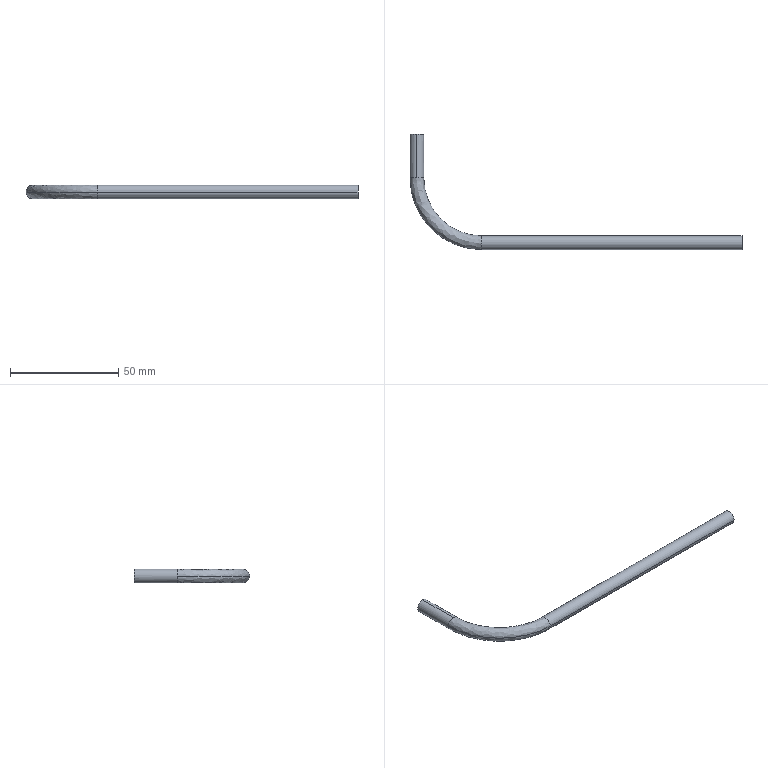Part | STEP file | copper tube 29_default_machined_ | 1 solid | 14 faces | box 153.175 x 53.175 x 6.35 mm | volume 2610 mm3 | cylinder 8 | spline 4 | plane 2 | commonest cylinder face diameters 4.75 x4 6.35 x4